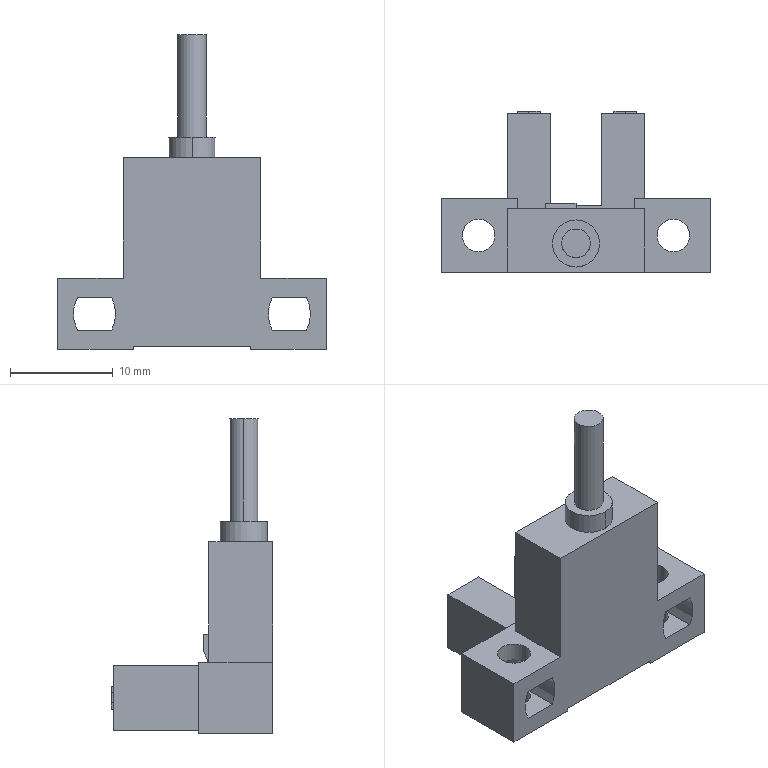Part | SolidWorks | features BaseBody 1 | 1 solid | 87 faces | box 26.2 x 15.7 x 30.7 mm | volume 2541 mm3 | plane 69 | cylinder 18 | commonest cylinder face diameters 3.2 x8 7 x6 2.8 x2 4.6 x2